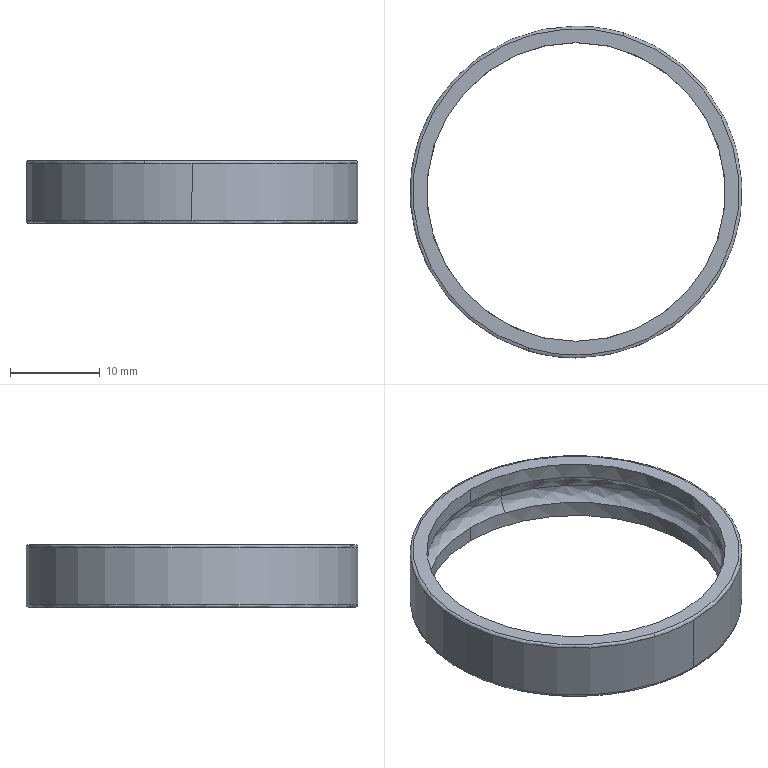Part | SolidWorks | features BaseBody 1 | 1 solid | 16 faces | box 37 x 37 x 7 mm | volume 1192 mm3 | spline 8 | cylinder 6 | plane 2 | commonest cylinder face diameters 33.3 x4 37 x2
STEP:
#1=CARTESIAN_POINT('',(518.571,7.238,245.844));
#2=VERTEX_POINT('',#1);
#3=CARTESIAN_POINT('',(513.262,8.017,245.844));
#4=VERTEX_POINT('',#3);
#5=CARTESIAN_POINT('',(513.262,-10.483,245.844));
#6=DIRECTION('',(0.000000004,-0.00000001,1.));
#7=DIRECTION('',(0.,-1.,-0.00000001));
#8=AXIS2_PLACEMENT_3D('',#5,#6,#7);
#9=CIRCLE('',#8,18.5);
#10=EDGE_CURVE('',#2,#4,#9,.T.);
#11=ORIENTED_EDGE('',*,*,#10,.F.);
#12=CARTESIAN_POINT('',(518.485,6.951,245.544));
#13=VERTEX_POINT('',#12);
#14=CARTESIAN_POINT('',(518.485,6.951,245.844));
#15=DIRECTION('',(-0.9579,0.287,0.000000007));
#16=DIRECTION('',(0.287,0.9579,0.000000008));
#17=AXIS2_PLACEMENT_3D('',#14,#15,#16);
#18=CIRCLE('',#17,0.3);
#19=EDGE_CURVE('',#2,#13,#18,.T.);
#20=ORIENTED_EDGE('',*,*,#19,.T.);
#21=CARTESIAN_POINT('',(508.038,-27.918,245.544));
#22=VERTEX_POINT('',#21);
#23=CARTESIAN_POINT('',(518.485,6.951,245.544));
#24=CARTESIAN_POINT('',(483.617,17.398,245.544));
#25=CARTESIAN_POINT('',(473.169,-17.47,245.544));
#26=CARTESIAN_POINT('',(508.038,-27.918,245.544));
#27=(BOUNDED_CURVE()B_SPLINE_CURVE(3,(#23,#24,#25,#26),.UNSPECIFIED.,.F.,.F.)B_SPLINE_CURVE_WITH_KNOTS((4,4),(0.,1.),.UNSPECIFIED.)CURVE()GEOMETRIC_REPRESENTATION_ITEM()RATIONAL_B_SPLINE_CURVE((1.,0.3333,0.3333,1.))REPRESENTATION_ITEM(''));
#28=EDGE_CURVE('',#13,#22,#27,.T.);
#29=ORIENTED_EDGE('',*,*,#28,.T.);
#30=CARTESIAN_POINT('',(507.952,-28.205,245.844));
#31=VERTEX_POINT('',#30);
#32=CARTESIAN_POINT('',(508.038,-27.918,245.844));
#33=DIRECTION('',(0.9579,-0.287,-0.000000007));
#34=DIRECTION('',(-0.287,-0.9579,-0.000000008));
#35=AXIS2_PLACEMENT_3D('',#32,#33,#34);
#36=CIRCLE('',#35,0.3);
#37=EDGE_CURVE('',#31,#22,#36,.T.);
#38=ORIENTED_EDGE('',*,*,#37,.F.);
#39=CARTESIAN_POINT('',(513.262,-10.483,245.844));
#40=DIRECTION('',(0.000000004,-0.00000001,1.));
#41=DIRECTION('',(0.,-1.,-0.00000001));
#42=AXIS2_PLACEMENT_3D('',#39,#40,#41);
#43=CIRCLE('',#42,18.5);
#44=EDGE_CURVE('',#4,#31,#43,.T.);
#45=ORIENTED_EDGE('',*,*,#44,.F.);
#46=EDGE_LOOP('',(#11,#20,#29,#38,#45));
#47=FACE_OUTER_BOUND('',#46,.T.);
#48=CARTESIAN_POINT('',(518.571,7.238,245.844));
#49=CARTESIAN_POINT('',(483.128,17.858,245.844));
#50=CARTESIAN_POINT('',(472.508,-17.585,245.844));
#51=CARTESIAN_POINT('',(507.952,-28.205,245.844));
#52=CARTESIAN_POINT('',(518.571,7.238,245.669));
#53=CARTESIAN_POINT('',(483.128,17.858,245.669));
#54=CARTESIAN_POINT('',(472.508,-17.585,245.669));
#55=CARTESIAN_POINT('',(507.952,-28.205,245.669));
#56=CARTESIAN_POINT('',(518.536,7.119,245.544));
#57=CARTESIAN_POINT('',(483.331,17.668,245.544));
#58=CARTESIAN_POINT('',(472.782,-17.537,245.544));
#59=CARTESIAN_POINT('',(507.987,-28.086,245.544));
#60=CARTESIAN_POINT('',(518.485,6.951,245.544));
#61=CARTESIAN_POINT('',(483.617,17.398,245.544));
#62=CARTESIAN_POINT('',(473.169,-17.47,245.544));
#63=CARTESIAN_POINT('',(508.038,-27.918,245.544));
#64=(BOUNDED_SURFACE()B_SPLINE_SURFACE(3,3,((#48,#49,#50,#51),(#52,#53,#54,#55),(#56,#57,#58,#59),(#60,#61,#62,#63)),.UNSPECIFIED.,.F.,.F.,.F.)B_SPLINE_SURFACE_WITH_KNOTS((4,4),(4,4),(0.,1.),(0.,1.),.UNSPECIFIED.)GEOMETRIC_REPRESENTATION_ITEM()RATIONAL_B_SPLINE_SURFACE(((1.,0.3333,0.3333,1.),(0.8047,0.2682,0.2682,0.8047),(0.8047,0.2682,0.2682,0.8047),(1.,0.3333,0.3333,1.)))REPRESENTATION_ITEM('')SURFACE());
#65=ADVANCED_FACE('',(#47),#64,.T.);
#66=CARTESIAN_POINT('',(508.038,-27.918,252.544));
#67=VERTEX_POINT('',#66);
#68=CARTESIAN_POINT('',(518.485,6.951,252.544));
#69=VERTEX_POINT('',#68);
#70=CARTESIAN_POINT('',(508.038,-27.918,252.544));
#71=CARTESIAN_POINT('',(473.169,-17.47,252.544));
#72=CARTESIAN_POINT('',(483.617,17.398,252.544));
#73=CARTESIAN_POINT('',(518.485,6.951,252.544));
#74=(BOUNDED_CURVE()B_SPLINE_CURVE(3,(#70,#71,#72,#73),.UNSPECIFIED.,.F.,.F.)B_SPLINE_CURVE_WITH_KNOTS((4,4),(0.,1.),.UNSPECIFIED.)CURVE()GEOMETRIC_REPRESENTATION_ITEM()RATIONAL_B_SPLINE_CURVE((1.,0.3333,0.3333,1.))REPRESENTATION_ITEM(''));
#75=EDGE_CURVE('',#67,#69,#74,.T.);
#76=ORIENTED_EDGE('',*,*,#75,.T.);
#77=CARTESIAN_POINT('',(518.571,7.238,252.244));
#78=VERTEX_POINT('',#77);
#79=CARTESIAN_POINT('',(518.485,6.951,252.244));
#80=DIRECTION('',(-0.9579,0.287,0.000000007));
#81=DIRECTION('',(0.287,0.9579,0.000000008));
#82=AXIS2_PLACEMENT_3D('',#79,#80,#81);
#83=CIRCLE('',#82,0.3);
#84=EDGE_CURVE('',#69,#78,#83,.T.);
#85=ORIENTED_EDGE('',*,*,#84,.T.);
#86=CARTESIAN_POINT('',(513.262,8.017,252.244));
#87=VERTEX_POINT('',#86);
#88=CARTESIAN_POINT('',(513.262,-10.483,252.244));
#89=DIRECTION('',(-0.000000004,0.00000001,-1.));
#90=DIRECTION('',(0.,-1.,-0.00000001));
#91=AXIS2_PLACEMENT_3D('',#88,#89,#90);
#92=CIRCLE('',#91,18.5);
#93=EDGE_CURVE('',#87,#78,#92,.T.);
#94=ORIENTED_EDGE('',*,*,#93,.F.);
#95=CARTESIAN_POINT('',(507.952,-28.205,252.244));
#96=VERTEX_POINT('',#95);
#97=CARTESIAN_POINT('',(513.262,-10.483,252.244));
#98=DIRECTION('',(-0.000000004,0.00000001,-1.));
#99=DIRECTION('',(0.,-1.,-0.00000001));
#100=AXIS2_PLACEMENT_3D('',#97,#98,#99);
#101=CIRCLE('',#100,18.5);
#102=EDGE_CURVE('',#96,#87,#101,.T.);
#103=ORIENTED_EDGE('',*,*,#102,.F.);
#104=CARTESIAN_POINT('',(508.038,-27.918,252.244));
#105=DIRECTION('',(0.9579,-0.287,-0.000000007));
#106=DIRECTION('',(-0.287,-0.9579,-0.000000008));
#107=AXIS2_PLACEMENT_3D('',#104,#105,#106);
#108=CIRCLE('',#107,0.3);
#109=EDGE_CURVE('',#67,#96,#108,.T.);
#110=ORIENTED_EDGE('',*,*,#109,.F.);
#111=EDGE_LOOP('',(#76,#85,#94,#103,#110));
#112=FACE_OUTER_BOUND('',#111,.T.);
#113=CARTESIAN_POINT('',(518.485,6.951,252.544));
#114=CARTESIAN_POINT('',(483.617,17.398,252.544));
#115=CARTESIAN_POINT('',(473.169,-17.47,252.544));
#116=CARTESIAN_POINT('',(508.038,-27.918,252.544));
#117=CARTESIAN_POINT('',(518.536,7.119,252.544));
#118=CARTESIAN_POINT('',(483.331,17.668,252.544));
#119=CARTESIAN_POINT('',(472.782,-17.537,252.544));
#120=CARTESIAN_POINT('',(507.987,-28.086,252.544));
#121=CARTESIAN_POINT('',(518.571,7.238,252.42));
#122=CARTESIAN_POINT('',(483.128,17.858,252.42));
#123=CARTESIAN_POINT('',(472.508,-17.585,252.42));
#124=CARTESIAN_POINT('',(507.952,-28.205,252.42));
#125=CARTESIAN_POINT('',(518.571,7.238,252.244));
#126=CARTESIAN_POINT('',(483.128,17.858,252.244));
#127=CARTESIAN_POINT('',(472.508,-17.585,252.244));
#128=CARTESIAN_POINT('',(507.952,-28.205,252.244));
#129=(BOUNDED_SURFACE()B_SPLINE_SURFACE(3,3,((#113,#114,#115,#116),(#117,#118,#119,#120),(#121,#122,#123,#124),(#125,#126,#127,#128)),.UNSPECIFIED.,.F.,.F.,.T.)B_SPLINE_SURFACE_WITH_KNOTS((4,4),(4,4),(0.,1.),(0.,1.),.UNSPECIFIED.)GEOMETRIC_REPRESENTATION_ITEM()RATIONAL_B_SPLINE_SURFACE(((1.,0.3333,0.3333,1.),(0.8047,0.2682,0.2682,0.8047),(0.8047,0.2682,0.2682,0.8047),(1.,0.3333,0.3333,1.)))REPRESENTATION_ITEM('')SURFACE());
#130=ADVANCED_FACE('',(#112),#129,.T.);
#131=CARTESIAN_POINT('',(513.262,-27.133,250.768));
#132=VERTEX_POINT('',#131);
#133=CARTESIAN_POINT('',(518.04,5.466,250.768));
#134=VERTEX_POINT('',#133);
#135=CARTESIAN_POINT('',(513.262,-10.483,250.768));
#136=DIRECTION('',(0.000000004,-0.00000001,1.));
#137=DIRECTION('',(0.,-1.,-0.00000001));
#138=AXIS2_PLACEMENT_3D('',#135,#136,#137);
#139=CIRCLE('',#138,16.65);
#140=EDGE_CURVE('',#132,#134,#139,.T.);
#141=ORIENTED_EDGE('',*,*,#140,.T.);
#142=CARTESIAN_POINT('',(518.299,6.328,249.044));
#143=VERTEX_POINT('',#142);
#144=CARTESIAN_POINT('',(517.696,4.317,249.044));
#145=DIRECTION('',(-0.9579,0.287,0.000000007));
#146=DIRECTION('',(0.287,0.9579,0.000000008));
#147=AXIS2_PLACEMENT_3D('',#144,#145,#146);
#148=CIRCLE('',#147,2.1);
#149=EDGE_CURVE('',#134,#143,#148,.T.);
#150=ORIENTED_EDGE('',*,*,#149,.T.);
#151=CARTESIAN_POINT('',(508.224,-27.295,249.044));
#152=VERTEX_POINT('',#151);
#153=CARTESIAN_POINT('',(513.262,-10.483,249.044));
#154=DIRECTION('',(0.000000004,-0.00000001,1.));
#155=DIRECTION('',(-0.287,-0.9579,-0.000000008));
#156=AXIS2_PLACEMENT_3D('',#153,#154,#155);
#157=CIRCLE('',#156,17.55);
#158=EDGE_CURVE('',#152,#143,#157,.T.);
#159=ORIENTED_EDGE('',*,*,#158,.F.);
#160=CARTESIAN_POINT('',(508.483,-26.433,250.768));
#161=VERTEX_POINT('',#160);
#162=CARTESIAN_POINT('',(508.827,-25.283,249.044));
#163=DIRECTION('',(0.9579,-0.287,-0.000000007));
#164=DIRECTION('',(-0.287,-0.9579,-0.000000008));
#165=AXIS2_PLACEMENT_3D('',#162,#163,#164);
#166=CIRCLE('',#165,2.1);
#167=EDGE_CURVE('',#161,#152,#166,.T.);
#168=ORIENTED_EDGE('',*,*,#167,.F.);
#169=CARTESIAN_POINT('',(513.262,-10.483,250.768));
#170=DIRECTION('',(0.000000004,-0.00000001,1.));
#171=DIRECTION('',(0.,-1.,-0.00000001));
#172=AXIS2_PLACEMENT_3D('',#169,#170,#171);
#173=CIRCLE('',#172,16.65);
#174=EDGE_CURVE('',#161,#132,#173,.T.);
#175=ORIENTED_EDGE('',*,*,#174,.T.);
#176=EDGE_LOOP('',(#141,#150,#159,#168,#175));
#177=FACE_OUTER_BOUND('',#176,.T.);
#178=CARTESIAN_POINT('',(508.483,-26.433,250.768));
#179=CARTESIAN_POINT('',(540.381,-35.991,250.768));
#180=CARTESIAN_POINT('',(549.939,-4.092,250.768));
#181=CARTESIAN_POINT('',(518.04,5.466,250.768));
#182=CARTESIAN_POINT('',(508.317,-26.984,250.367));
#183=CARTESIAN_POINT('',(541.319,-36.872,250.367));
#184=CARTESIAN_POINT('',(551.207,-3.871,250.367));
#185=CARTESIAN_POINT('',(518.206,6.017,250.367));
#186=CARTESIAN_POINT('',(508.224,-27.295,249.745));
#187=CARTESIAN_POINT('',(541.847,-37.369,249.745));
#188=CARTESIAN_POINT('',(551.922,-3.746,249.745));
#189=CARTESIAN_POINT('',(518.299,6.328,249.745));
#190=CARTESIAN_POINT('',(508.224,-27.295,249.044));
#191=CARTESIAN_POINT('',(541.847,-37.369,249.044));
#192=CARTESIAN_POINT('',(551.922,-3.746,249.044));
#193=CARTESIAN_POINT('',(518.299,6.328,249.044));
#194=(BOUNDED_SURFACE()B_SPLINE_SURFACE(3,3,((#178,#179,#180,#181),(#182,#183,#184,#185),(#186,#187,#188,#189),(#190,#191,#192,#193)),.UNSPECIFIED.,.F.,.F.,.F.)B_SPLINE_SURFACE_WITH_KNOTS((4,4),(4,4),(0.,1.),(0.,1.),.UNSPECIFIED.)GEOMETRIC_REPRESENTATION_ITEM()RATIONAL_B_SPLINE_SURFACE(((1.,0.3333,0.3333,1.),(0.9243,0.3081,0.3081,0.9243),(0.9243,0.3081,0.3081,0.9243),(1.,0.3333,0.3333,1.)))REPRESENTATION_ITEM('')SURFACE());
#195=ADVANCED_FACE('',(#177),#194,.F.);
#196=ORIENTED_EDGE('',*,*,#158,.T.);
#197=CARTESIAN_POINT('',(518.04,5.466,247.321));
#198=VERTEX_POINT('',#197);
#199=CARTESIAN_POINT('',(517.696,4.317,249.044));
#200=DIRECTION('',(-0.9579,0.287,0.000000007));
#201=DIRECTION('',(0.287,0.9579,0.000000008));
#202=AXIS2_PLACEMENT_3D('',#199,#200,#201);
#203=CIRCLE('',#202,2.1);
#204=EDGE_CURVE('',#143,#198,#203,.T.);
#205=ORIENTED_EDGE('',*,*,#204,.T.);
#206=CARTESIAN_POINT('',(513.262,-27.133,247.321));
#207=VERTEX_POINT('',#206);
#208=CARTESIAN_POINT('',(513.262,-10.483,247.321));
#209=DIRECTION('',(-0.000000004,0.00000001,-1.));
#210=DIRECTION('',(0.,-1.,-0.00000001));
#211=AXIS2_PLACEMENT_3D('',#208,#209,#210);
#212=CIRCLE('',#211,16.65);
#213=EDGE_CURVE('',#198,#207,#212,.T.);
#214=ORIENTED_EDGE('',*,*,#213,.T.);
#215=CARTESIAN_POINT('',(508.483,-26.433,247.321));
#216=VERTEX_POINT('',#215);
#217=CARTESIAN_POINT('',(513.262,-10.483,247.321));
#218=DIRECTION('',(-0.000000004,0.00000001,-1.));
#219=DIRECTION('',(0.,-1.,-0.00000001));
#220=AXIS2_PLACEMENT_3D('',#217,#218,#219);
#221=CIRCLE('',#220,16.65);
#222=EDGE_CURVE('',#207,#216,#221,.T.);
#223=ORIENTED_EDGE('',*,*,#222,.T.);
#224=CARTESIAN_POINT('',(508.827,-25.283,249.044));
#225=DIRECTION('',(0.9579,-0.287,-0.000000007));
#226=DIRECTION('',(-0.287,-0.9579,-0.000000008));
#227=AXIS2_PLACEMENT_3D('',#224,#225,#226);
#228=CIRCLE('',#227,2.1);
#229=EDGE_CURVE('',#152,#216,#228,.T.);
#230=ORIENTED_EDGE('',*,*,#229,.F.);
#231=EDGE_LOOP('',(#196,#205,#214,#223,#230));
#232=FACE_OUTER_BOUND('',#231,.T.);
#233=CARTESIAN_POINT('',(508.224,-27.295,249.044));
#234=CARTESIAN_POINT('',(541.847,-37.369,249.044));
#235=CARTESIAN_POINT('',(551.922,-3.746,249.044));
#236=CARTESIAN_POINT('',(518.299,6.328,249.044));
#237=CARTESIAN_POINT('',(508.224,-27.295,248.343));
#238=CARTESIAN_POINT('',(541.847,-37.369,248.343));
#239=CARTESIAN_POINT('',(551.922,-3.746,248.343));
#240=CARTESIAN_POINT('',(518.299,6.328,248.343));
#241=CARTESIAN_POINT('',(508.317,-26.984,247.722));
#242=CARTESIAN_POINT('',(541.319,-36.872,247.722));
#243=CARTESIAN_POINT('',(551.207,-3.871,247.722));
#244=CARTESIAN_POINT('',(518.206,6.017,247.722));
#245=CARTESIAN_POINT('',(508.483,-26.433,247.321));
#246=CARTESIAN_POINT('',(540.381,-35.991,247.321));
#247=CARTESIAN_POINT('',(549.939,-4.092,247.321));
#248=CARTESIAN_POINT('',(518.04,5.466,247.321));
#249=(BOUNDED_SURFACE()B_SPLINE_SURFACE(3,3,((#233,#234,#235,#236),(#237,#238,#239,#240),(#241,#242,#243,#244),(#245,#246,#247,#248)),.UNSPECIFIED.,.F.,.F.,.F.)B_SPLINE_SURFACE_WITH_KNOTS((4,4),(4,4),(0.,1.),(0.,1.),.UNSPECIFIED.)GEOMETRIC_REPRESENTATION_ITEM()RATIONAL_B_SPLINE_SURFACE(((1.,0.3333,0.3333,1.),(0.9243,0.3081,0.3081,0.9243),(0.9243,0.3081,0.3081,0.9243),(1.,0.3333,0.3333,1.)))REPRESENTATION_ITEM('')SURFACE());
#250=ADVANCED_FACE('',(#232),#249,.F.);
#251=CARTESIAN_POINT('',(513.262,-28.983,245.844));
#252=VERTEX_POINT('',#251);
#253=CARTESIAN_POINT('',(513.262,-10.483,245.844));
#254=DIRECTION('',(0.000000004,-0.00000001,1.));
#255=DIRECTION('',(0.,-1.,-0.00000001));
#256=AXIS2_PLACEMENT_3D('',#253,#254,#255);
#257=CIRCLE('',#256,18.5);
#258=EDGE_CURVE('',#252,#2,#257,.T.);
#259=ORIENTED_EDGE('',*,*,#258,.T.);
#260=ORIENTED_EDGE('',*,*,#10,.T.);
#261=CARTESIAN_POINT('',(513.262,8.017,249.044));
#262=DIRECTION('',(0.000000004,-0.00000001,1.));
#263=VECTOR('',#262,1000.);
#264=LINE('',#261,#263);
#265=EDGE_CURVE('',#4,#87,#264,.T.);
#266=ORIENTED_EDGE('',*,*,#265,.T.);
#267=ORIENTED_EDGE('',*,*,#93,.T.);
#268=CARTESIAN_POINT('',(513.262,-28.983,252.244));
#269=VERTEX_POINT('',#268);
#270=CARTESIAN_POINT('',(513.262,-10.483,252.244));
#271=DIRECTION('',(-0.000000004,0.00000001,-1.));
#272=DIRECTION('',(0.,-1.,-0.00000001));
#273=AXIS2_PLACEMENT_3D('',#270,#271,#272);
#274=CIRCLE('',#273,18.5);
#275=EDGE_CURVE('',#78,#269,#274,.T.);
#276=ORIENTED_EDGE('',*,*,#275,.T.);
#277=CARTESIAN_POINT('',(513.262,-28.983,249.044));
#278=DIRECTION('',(0.000000004,-0.00000001,1.));
#279=VECTOR('',#278,1000.);
#280=LINE('',#277,#279);
#281=EDGE_CURVE('',#252,#269,#280,.T.);
#282=ORIENTED_EDGE('',*,*,#281,.F.);
#283=EDGE_LOOP('',(#259,#260,#266,#267,#276,#282));
#284=FACE_OUTER_BOUND('',#283,.T.);
#285=CARTESIAN_POINT('',(513.262,-10.483,249.044));
#286=DIRECTION('',(0.000000004,-0.00000001,1.));
#287=DIRECTION('',(0.,-1.,-0.00000001));
#288=AXIS2_PLACEMENT_3D('',#285,#286,#287);
#289=CYLINDRICAL_SURFACE('',#288,18.5);
#290=ADVANCED_FACE('',(#284),#289,.T.);
#291=CARTESIAN_POINT('',(513.262,6.167,245.544));
#292=VERTEX_POINT('',#291);
#293=CARTESIAN_POINT('',(513.262,-27.133,245.544));
#294=VERTEX_POINT('',#293);
#295=CARTESIAN_POINT('',(513.262,-10.483,245.544));
#296=DIRECTION('',(0.000000004,-0.00000001,1.));
#297=DIRECTION('',(0.,-1.,-0.00000001));
#298=AXIS2_PLACEMENT_3D('',#295,#296,#297);
#299=CIRCLE('',#298,16.65);
#300=EDGE_CURVE('',#292,#294,#299,.T.);
#301=ORIENTED_EDGE('',*,*,#300,.F.);
#302=CARTESIAN_POINT('',(513.262,6.167,247.321));
#303=VERTEX_POINT('',#302);
#304=CARTESIAN_POINT('',(513.262,6.167,246.433));
#305=DIRECTION('',(0.000000004,-0.00000001,1.));
#306=VECTOR('',#305,1000.);
#307=LINE('',#304,#306);
#308=EDGE_CURVE('',#292,#303,#307,.T.);
#309=ORIENTED_EDGE('',*,*,#308,.T.);
#310=CARTESIAN_POINT('',(513.262,-10.483,247.321));
#311=DIRECTION('',(-0.000000004,0.00000001,-1.));
#312=DIRECTION('',(0.,-1.,-0.00000001));
#313=AXIS2_PLACEMENT_3D('',#310,#311,#312);
#314=CIRCLE('',#313,16.65);
#315=EDGE_CURVE('',#216,#303,#314,.T.);
#316=ORIENTED_EDGE('',*,*,#315,.F.);
#317=ORIENTED_EDGE('',*,*,#222,.F.);
#318=CARTESIAN_POINT('',(513.262,-27.133,246.433));
#319=DIRECTION('',(0.000000004,-0.00000001,1.));
#320=VECTOR('',#319,1000.);
#321=LINE('',#318,#320);
#322=EDGE_CURVE('',#294,#207,#321,.T.);
#323=ORIENTED_EDGE('',*,*,#322,.F.);
#324=EDGE_LOOP('',(#301,#309,#316,#317,#323));
#325=FACE_OUTER_BOUND('',#324,.T.);
#326=CARTESIAN_POINT('',(513.262,-10.483,246.433));
#327=DIRECTION('',(0.000000004,-0.00000001,1.));
#328=DIRECTION('',(0.,-1.,-0.00000001));
#329=AXIS2_PLACEMENT_3D('',#326,#327,#328);
#330=CYLINDRICAL_SURFACE('',#329,16.65);
#331=ADVANCED_FACE('',(#325),#330,.F.);
#332=CARTESIAN_POINT('',(513.262,6.167,250.768));
#333=VERTEX_POINT('',#332);
#334=CARTESIAN_POINT('',(513.262,-10.483,250.768));
#335=DIRECTION('',(0.000000004,-0.00000001,1.));
#336=DIRECTION('',(0.,-1.,-0.00000001));
#337=AXIS2_PLACEMENT_3D('',#334,#335,#336);
#338=CIRCLE('',#337,16.65);
#339=EDGE_CURVE('',#333,#161,#338,.T.);
#340=ORIENTED_EDGE('',*,*,#339,.F.);
#341=CARTESIAN_POINT('',(513.262,6.167,252.544));
#342=VERTEX_POINT('',#341);
#343=CARTESIAN_POINT('',(513.262,6.167,251.656));
#344=DIRECTION('',(0.000000004,-0.00000001,1.));
#345=VECTOR('',#344,1000.);
#346=LINE('',#343,#345);
#347=EDGE_CURVE('',#333,#342,#346,.T.);
#348=ORIENTED_EDGE('',*,*,#347,.T.);
#349=CARTESIAN_POINT('',(513.262,-27.133,252.544));
#350=VERTEX_POINT('',#349);
#351=CARTESIAN_POINT('',(513.262,-10.483,252.544));
#352=DIRECTION('',(-0.000000004,0.00000001,-1.));
#353=DIRECTION('',(0.,-1.,-0.00000001));
#354=AXIS2_PLACEMENT_3D('',#351,#352,#353);
#355=CIRCLE('',#354,16.65);
#356=EDGE_CURVE('',#350,#342,#355,.T.);
#357=ORIENTED_EDGE('',*,*,#356,.F.);
#358=CARTESIAN_POINT('',(513.262,-27.133,251.656));
#359=DIRECTION('',(0.000000004,-0.00000001,1.));
#360=VECTOR('',#359,1000.);
#361=LINE('',#358,#360);
#362=EDGE_CURVE('',#132,#350,#361,.T.);
#363=ORIENTED_EDGE('',*,*,#362,.F.);
#364=ORIENTED_EDGE('',*,*,#174,.F.);
#365=EDGE_LOOP('',(#340,#348,#357,#363,#364));
#366=FACE_OUTER_BOUND('',#365,.T.);
#367=CARTESIAN_POINT('',(513.262,-10.483,251.656));
#368=DIRECTION('',(0.000000004,-0.00000001,1.));
#369=DIRECTION('',(0.,-1.,-0.00000001));
#370=AXIS2_PLACEMENT_3D('',#367,#368,#369);
#371=CYLINDRICAL_SURFACE('',#370,16.65);
#372=ADVANCED_FACE('',(#366),#371,.F.);
#373=ORIENTED_EDGE('',*,*,#204,.F.);
#374=CARTESIAN_POINT('',(513.262,-10.483,249.044));
#375=DIRECTION('',(0.000000004,-0.00000001,1.));
#376=DIRECTION('',(-0.287,-0.9579,-0.000000008));
#377=AXIS2_PLACEMENT_3D('',#374,#375,#376);
#378=CIRCLE('',#377,17.55);
#379=EDGE_CURVE('',#143,#152,#378,.T.);
#380=ORIENTED_EDGE('',*,*,#379,.T.);
#381=ORIENTED_EDGE('',*,*,#229,.T.);
#382=ORIENTED_EDGE('',*,*,#315,.T.);
#383=CARTESIAN_POINT('',(513.262,-10.483,247.321));
#384=DIRECTION('',(-0.000000004,0.00000001,-1.));
#385=DIRECTION('',(0.,-1.,-0.00000001));
#386=AXIS2_PLACEMENT_3D('',#383,#384,#385);
#387=CIRCLE('',#386,16.65);
#388=EDGE_CURVE('',#303,#198,#387,.T.);
#389=ORIENTED_EDGE('',*,*,#388,.T.);
#390=EDGE_LOOP('',(#373,#380,#381,#382,#389));
#391=FACE_OUTER_BOUND('',#390,.T.);
#392=CARTESIAN_POINT('',(518.299,6.328,249.044));
#393=CARTESIAN_POINT('',(484.676,16.403,249.044));
#394=CARTESIAN_POINT('',(474.601,-17.22,249.044));
#395=CARTESIAN_POINT('',(508.224,-27.295,249.044));
#396=CARTESIAN_POINT('',(518.299,6.328,248.343));
#397=CARTESIAN_POINT('',(484.676,16.403,248.343));
#398=CARTESIAN_POINT('',(474.601,-17.22,248.343));
#399=CARTESIAN_POINT('',(508.224,-27.295,248.343));
#400=CARTESIAN_POINT('',(518.206,6.017,247.722));
#401=CARTESIAN_POINT('',(485.204,15.905,247.722));
#402=CARTESIAN_POINT('',(475.316,-17.096,247.722));
#403=CARTESIAN_POINT('',(508.317,-26.984,247.722));
#404=CARTESIAN_POINT('',(518.04,5.466,247.321));
#405=CARTESIAN_POINT('',(486.142,15.024,247.321));
#406=CARTESIAN_POINT('',(476.584,-16.875,247.321));
#407=CARTESIAN_POINT('',(508.483,-26.433,247.321));
#408=(BOUNDED_SURFACE()B_SPLINE_SURFACE(3,3,((#392,#393,#394,#395),(#396,#397,#398,#399),(#400,#401,#402,#403),(#404,#405,#406,#407)),.UNSPECIFIED.,.F.,.F.,.F.)B_SPLINE_SURFACE_WITH_KNOTS((4,4),(4,4),(0.,1.),(0.,1.),.UNSPECIFIED.)GEOMETRIC_REPRESENTATION_ITEM()RATIONAL_B_SPLINE_SURFACE(((1.,0.3333,0.3333,1.),(0.9243,0.3081,0.3081,0.9243),(0.9243,0.3081,0.3081,0.9243),(1.,0.3333,0.3333,1.)))REPRESENTATION_ITEM('')SURFACE());
#409=ADVANCED_FACE('',(#391),#408,.F.);
#410=ORIENTED_EDGE('',*,*,#265,.F.);
#411=ORIENTED_EDGE('',*,*,#44,.T.);
#412=CARTESIAN_POINT('',(513.262,-10.483,245.844));
#413=DIRECTION('',(0.000000004,-0.00000001,1.));
#414=DIRECTION('',(0.,-1.,-0.00000001));
#415=AXIS2_PLACEMENT_3D('',#412,#413,#414);
#416=CIRCLE('',#415,18.5);
#417=EDGE_CURVE('',#31,#252,#416,.T.);
#418=ORIENTED_EDGE('',*,*,#417,.T.);
#419=ORIENTED_EDGE('',*,*,#281,.T.);
#420=CARTESIAN_POINT('',(513.262,-10.483,252.244));
#421=DIRECTION('',(-0.000000004,0.00000001,-1.));
#422=DIRECTION('',(0.,-1.,-0.00000001));
#423=AXIS2_PLACEMENT_3D('',#420,#421,#422);
#424=CIRCLE('',#423,18.5);
#425=EDGE_CURVE('',#269,#96,#424,.T.);
#426=ORIENTED_EDGE('',*,*,#425,.T.);
#427=ORIENTED_EDGE('',*,*,#102,.T.);
#428=EDGE_LOOP('',(#410,#411,#418,#419,#426,#427));
#429=FACE_OUTER_BOUND('',#428,.T.);
#430=CARTESIAN_POINT('',(513.262,-10.483,249.044));
#431=DIRECTION('',(0.000000004,-0.00000001,1.));
#432=DIRECTION('',(0.,-1.,-0.00000001));
#433=AXIS2_PLACEMENT_3D('',#430,#431,#432);
#434=CYLINDRICAL_SURFACE('',#433,18.5);
#435=ADVANCED_FACE('',(#429),#434,.T.);
#436=ORIENTED_EDGE('',*,*,#19,.F.);
#437=ORIENTED_EDGE('',*,*,#258,.F.);
#438=ORIENTED_EDGE('',*,*,#417,.F.);
#439=ORIENTED_EDGE('',*,*,#37,.T.);
#440=CARTESIAN_POINT('',(518.485,6.951,245.544));
#441=CARTESIAN_POINT('',(519.018,6.791,245.544));
#442=CARTESIAN_POINT('',(519.804,6.516,245.544));
#443=CARTESIAN_POINT('',(520.695,6.133,245.544));
#444=CARTESIAN_POINT('',(521.135,5.926,245.544));
#445=CARTESIAN_POINT('',(521.353,5.819,245.544));
#446=CARTESIAN_POINT('',(521.446,5.772,245.544));
#447=CARTESIAN_POINT('',(521.509,5.741,245.544));
#448=CARTESIAN_POINT('',(521.538,5.726,245.544));
#449=CARTESIAN_POINT('',(522.095,5.44,245.544));
#450=CARTESIAN_POINT('',(522.86,5.,245.544));
#451=CARTESIAN_POINT('',(523.711,4.423,245.544));
#452=CARTESIAN_POINT('',(524.127,4.119,245.544));
#453=CARTESIAN_POINT('',(524.332,3.963,245.544));
#454=CARTESIAN_POINT('',(524.42,3.895,245.544));
#455=CARTESIAN_POINT('',(524.478,3.85,245.544));
#456=CARTESIAN_POINT('',(524.506,3.828,245.544));
#457=CARTESIAN_POINT('',(525.019,3.423,245.544));
#458=CARTESIAN_POINT('',(525.71,2.818,245.544));
#459=CARTESIAN_POINT('',(526.461,2.054,245.544));
#460=CARTESIAN_POINT('',(526.822,1.657,245.544));
#461=CARTESIAN_POINT('',(526.974,1.484,245.544));
#462=CARTESIAN_POINT('',(527.074,1.368,245.544));
#463=CARTESIAN_POINT('',(527.123,1.311,245.544));
#464=CARTESIAN_POINT('',(527.984,0.2903,245.544));
#465=CARTESIAN_POINT('',(528.687,-0.7435,245.544));
#466=CARTESIAN_POINT('',(529.581,-2.402,245.544));
#467=CARTESIAN_POINT('',(529.983,-3.25,245.544));
#468=CARTESIAN_POINT('',(530.374,-4.272,245.544));
#469=CARTESIAN_POINT('',(530.55,-4.791,245.544));
#470=CARTESIAN_POINT('',(530.621,-5.015,245.544));
#471=CARTESIAN_POINT('',(530.667,-5.165,245.544));
#472=CARTESIAN_POINT('',(530.691,-5.242,245.544));
#473=CARTESIAN_POINT('',(530.887,-5.905,245.544));
#474=CARTESIAN_POINT('',(531.103,-6.798,245.544));
#475=CARTESIAN_POINT('',(531.276,-7.855,245.544));
#476=CARTESIAN_POINT('',(531.342,-8.388,245.544));
#477=CARTESIAN_POINT('',(531.37,-8.655,245.544));
#478=CARTESIAN_POINT('',(531.381,-8.77,245.544));
#479=CARTESIAN_POINT('',(531.388,-8.846,245.544));
#480=CARTESIAN_POINT('',(531.391,-8.886,245.544));
#481=CARTESIAN_POINT('',(531.445,-9.511,245.544));
#482=CARTESIAN_POINT('',(531.478,-10.392,245.544));
#483=CARTESIAN_POINT('',(531.442,-11.42,245.544));
#484=CARTESIAN_POINT('',(531.405,-11.934,245.544));
#485=CARTESIAN_POINT('',(531.382,-12.191,245.544));
#486=CARTESIAN_POINT('',(531.371,-12.301,245.544));
#487=CARTESIAN_POINT('',(531.363,-12.374,245.544));
#488=CARTESIAN_POINT('',(531.359,-12.413,245.544));
#489=CARTESIAN_POINT('',(531.235,-13.554,245.544));
#490=CARTESIAN_POINT('',(531.015,-14.641,245.544));
#491=CARTESIAN_POINT('',(530.536,-16.24,245.544));
#492=CARTESIAN_POINT('',(530.261,-17.026,245.544));
#493=CARTESIAN_POINT('',(529.878,-17.917,245.544));
#494=CARTESIAN_POINT('',(529.671,-18.357,245.544));
#495=CARTESIAN_POINT('',(529.564,-18.575,245.544));
#496=CARTESIAN_POINT('',(529.517,-18.668,245.544));
#497=CARTESIAN_POINT('',(529.486,-18.73,245.544));
#498=CARTESIAN_POINT('',(529.471,-18.76,245.544));
#499=CARTESIAN_POINT('',(529.185,-19.317,245.544));
#500=CARTESIAN_POINT('',(528.745,-20.082,245.544));
#501=CARTESIAN_POINT('',(528.168,-20.933,245.544));
#502=CARTESIAN_POINT('',(527.864,-21.349,245.544));
#503=CARTESIAN_POINT('',(527.708,-21.554,245.544));
#504=CARTESIAN_POINT('',(527.64,-21.642,245.544));
#505=CARTESIAN_POINT('',(527.594,-21.7,245.544));
#506=CARTESIAN_POINT('',(527.573,-21.728,245.544));
#507=CARTESIAN_POINT('',(527.168,-22.241,245.544));
#508=CARTESIAN_POINT('',(526.563,-22.932,245.544));
#509=CARTESIAN_POINT('',(525.799,-23.683,245.544));
#510=CARTESIAN_POINT('',(525.402,-24.044,245.544));
#511=CARTESIAN_POINT('',(525.229,-24.196,245.544));
#512=CARTESIAN_POINT('',(525.113,-24.296,245.544));
#513=CARTESIAN_POINT('',(525.055,-24.345,245.544));
#514=CARTESIAN_POINT('',(524.035,-25.206,245.544));
#515=CARTESIAN_POINT('',(523.001,-25.909,245.544));
#516=CARTESIAN_POINT('',(521.343,-26.803,245.544));
#517=CARTESIAN_POINT('',(520.495,-27.205,245.544));
#518=CARTESIAN_POINT('',(519.473,-27.596,245.544));
#519=CARTESIAN_POINT('',(518.954,-27.772,245.544));
#520=CARTESIAN_POINT('',(518.73,-27.843,245.544));
#521=CARTESIAN_POINT('',(518.58,-27.889,245.544));
#522=CARTESIAN_POINT('',(518.503,-27.912,245.544));
#523=CARTESIAN_POINT('',(517.84,-28.109,245.544));
#524=CARTESIAN_POINT('',(516.947,-28.325,245.544));
#525=CARTESIAN_POINT('',(515.889,-28.497,245.544));
#526=CARTESIAN_POINT('',(515.357,-28.564,245.544));
#527=CARTESIAN_POINT('',(515.09,-28.592,245.544));
#528=CARTESIAN_POINT('',(514.975,-28.603,245.544));
#529=CARTESIAN_POINT('',(514.899,-28.61,245.544));
#530=CARTESIAN_POINT('',(514.859,-28.613,245.544));
#531=CARTESIAN_POINT('',(514.234,-28.667,245.544));
#532=CARTESIAN_POINT('',(513.353,-28.7,245.544));
#533=CARTESIAN_POINT('',(512.325,-28.664,245.544));
#534=CARTESIAN_POINT('',(511.811,-28.627,245.544));
#535=CARTESIAN_POINT('',(511.554,-28.603,245.544));
#536=CARTESIAN_POINT('',(511.444,-28.592,245.544));
#537=CARTESIAN_POINT('',(511.371,-28.585,245.544));
#538=CARTESIAN_POINT('',(511.332,-28.581,245.544));
#539=CARTESIAN_POINT('',(510.191,-28.457,245.544));
#540=CARTESIAN_POINT('',(509.104,-28.237,245.544));
#541=CARTESIAN_POINT('',(508.038,-27.918,245.544));
#542=B_SPLINE_CURVE_WITH_KNOTS('',3,(#440,#441,#442,#443,#444,#445,#446,#447,#448,#449,#450,#451,#452,#453,#454,#455,#456,#457,#458,#459,#460,#461,#462,#463,#464,#465,#466,#467,#468,#469,#470,#471,#472,#473,#474,#475,#476,#477,#478,#479,#480,#481,#482,#483,#484,#485,#486,#487,#488,#489,#490,#491,#492,#493,#494,#495,#496,#497,#498,#499,#500,#501,#502,#503,#504,#505,#506,#507,#508,#509,#510,#511,#512,#513,#514,#515,#516,#517,#518,#519,#520,#521,#522,#523,#524,#525,#526,#527,#528,#529,#530,#531,#532,#533,#534,#535,#536,#537,#538,#539,#540,#541),.UNSPECIFIED.,.F.,.F.,(4,1,1,1,1,2,2,1,1,1,1,2,2,1,1,1,2,2,2,1,1,1,2,2,1,1,1,1,2,2,1,1,1,1,2,2,2,1,1,1,1,2,2,1,1,1,1,2,2,1,1,1,2,2,2,1,1,1,2,2,1,1,1,1,2,2,1,1,1,1,2,2,4),(0.,0.03125,0.04687,0.05469,0.05859,0.06055,0.0625,0.09375,0.1094,0.1172,0.1211,0.123,0.125,0.1563,0.1719,0.1797,0.1836,0.1875,0.25,0.2813,0.2969,0.3047,0.3086,0.3125,0.3438,0.3594,0.3672,0.3711,0.373,0.375,0.4063,0.4219,0.4297,0.4336,0.4355,0.4375,0.5,0.5313,0.5469,0.5547,0.5586,0.5605,0.5625,0.5938,0.6094,0.6172,0.6211,0.623,0.625,0.6563,0.6719,0.6797,0.6836,0.6875,0.75,0.7813,0.7969,0.8047,0.8086,0.8125,0.8438,0.8594,0.8672,0.8711,0.873,0.875,0.9063,0.9219,0.9297,0.9336,0.9355,0.9375,1.),.UNSPECIFIED.);
#543=EDGE_CURVE('',#13,#22,#542,.T.);
#544=ORIENTED_EDGE('',*,*,#543,.F.);
#545=EDGE_LOOP('',(#436,#437,#438,#439,#544));
#546=FACE_OUTER_BOUND('',#545,.T.);
#547=CARTESIAN_POINT('',(507.952,-28.205,245.844));
#548=CARTESIAN_POINT('',(543.395,-38.825,245.844));
#549=CARTESIAN_POINT('',(554.015,-3.382,245.844));
#550=CARTESIAN_POINT('',(518.571,7.238,245.844));
#551=CARTESIAN_POINT('',(507.952,-28.205,245.669));
#552=CARTESIAN_POINT('',(543.395,-38.825,245.669));
#553=CARTESIAN_POINT('',(554.015,-3.382,245.669));
#554=CARTESIAN_POINT('',(518.571,7.238,245.669));
#555=CARTESIAN_POINT('',(507.987,-28.086,245.544));
#556=CARTESIAN_POINT('',(543.192,-38.634,245.544));
#557=CARTESIAN_POINT('',(553.741,-3.429,245.544));
#558=CARTESIAN_POINT('',(518.536,7.119,245.544));
#559=CARTESIAN_POINT('',(508.038,-27.918,245.544));
#560=CARTESIAN_POINT('',(542.906,-38.365,245.544));
#561=CARTESIAN_POINT('',(553.354,-3.497,245.544));
#562=CARTESIAN_POINT('',(518.485,6.951,245.544));
#563=(BOUNDED_SURFACE()B_SPLINE_SURFACE(3,3,((#547,#548,#549,#550),(#551,#552,#553,#554),(#555,#556,#557,#558),(#559,#560,#561,#562)),.UNSPECIFIED.,.F.,.F.,.F.)B_SPLINE_SURFACE_WITH_KNOTS((4,4),(4,4),(0.,1.),(0.,1.),.UNSPECIFIED.)GEOMETRIC_REPRESENTATION_ITEM()RATIONAL_B_SPLINE_SURFACE(((1.,0.3333,0.3333,1.),(0.8047,0.2682,0.2682,0.8047),(0.8047,0.2682,0.2682,0.8047),(1.,0.3333,0.3333,1.)))REPRESENTATION_ITEM('')SURFACE());
#564=ADVANCED_FACE('',(#546),#563,.T.);
#565=ORIENTED_EDGE('',*,*,#84,.F.);
#566=CARTESIAN_POINT('',(518.485,6.951,252.544));
#567=CARTESIAN_POINT('',(553.354,-3.497,252.544));
#568=CARTESIAN_POINT('',(542.906,-38.365,252.544));
#569=CARTESIAN_POINT('',(508.038,-27.918,252.544));
#570=(BOUNDED_CURVE()B_SPLINE_CURVE(3,(#566,#567,#568,#569),.UNSPECIFIED.,.F.,.F.)B_SPLINE_CURVE_WITH_KNOTS((4,4),(0.,1.),.UNSPECIFIED.)CURVE()GEOMETRIC_REPRESENTATION_ITEM()RATIONAL_B_SPLINE_CURVE((1.,0.3333,0.3333,1.))REPRESENTATION_ITEM(''));
#571=EDGE_CURVE('',#69,#67,#570,.T.);
#572=ORIENTED_EDGE('',*,*,#571,.T.);
#573=ORIENTED_EDGE('',*,*,#109,.T.);
#574=ORIENTED_EDGE('',*,*,#425,.F.);
#575=ORIENTED_EDGE('',*,*,#275,.F.);
#576=EDGE_LOOP('',(#565,#572,#573,#574,#575));
#577=FACE_OUTER_BOUND('',#576,.T.);
#578=CARTESIAN_POINT('',(508.038,-27.918,252.544));
#579=CARTESIAN_POINT('',(542.906,-38.365,252.544));
#580=CARTESIAN_POINT('',(553.354,-3.497,252.544));
#581=CARTESIAN_POINT('',(518.485,6.951,252.544));
#582=CARTESIAN_POINT('',(507.987,-28.086,252.544));
#583=CARTESIAN_POINT('',(543.192,-38.634,252.544));
#584=CARTESIAN_POINT('',(553.741,-3.429,252.544));
#585=CARTESIAN_POINT('',(518.536,7.119,252.544));
#586=CARTESIAN_POINT('',(507.952,-28.205,252.42));
#587=CARTESIAN_POINT('',(543.395,-38.825,252.42));
#588=CARTESIAN_POINT('',(554.015,-3.382,252.42));
#589=CARTESIAN_POINT('',(518.571,7.238,252.42));
#590=CARTESIAN_POINT('',(507.952,-28.205,252.244));
#591=CARTESIAN_POINT('',(543.395,-38.825,252.244));
#592=CARTESIAN_POINT('',(554.015,-3.382,252.244));
#593=CARTESIAN_POINT('',(518.571,7.238,252.244));
#594=(BOUNDED_SURFACE()B_SPLINE_SURFACE(3,3,((#578,#579,#580,#581),(#582,#583,#584,#585),(#586,#587,#588,#589),(#590,#591,#592,#593)),.UNSPECIFIED.,.F.,.F.,.F.)B_SPLINE_SURFACE_WITH_KNOTS((4,4),(4,4),(0.,1.),(0.,1.),.UNSPECIFIED.)GEOMETRIC_REPRESENTATION_ITEM()RATIONAL_B_SPLINE_SURFACE(((1.,0.3333,0.3333,1.),(0.8047,0.2682,0.2682,0.8047),(0.8047,0.2682,0.2682,0.8047),(1.,0.3333,0.3333,1.)))REPRESENTATION_ITEM('')SURFACE());
#595=ADVANCED_FACE('',(#577),#594,.T.);
#596=ORIENTED_EDGE('',*,*,#28,.F.);
#597=ORIENTED_EDGE('',*,*,#543,.T.);
#598=EDGE_LOOP('',(#596,#597));
#599=FACE_OUTER_BOUND('',#598,.T.);
#600=CARTESIAN_POINT('',(513.262,-10.483,245.544));
#601=DIRECTION('',(0.000000004,-0.00000001,1.));
#602=DIRECTION('',(0.,-1.,-0.00000001));
#603=AXIS2_PLACEMENT_3D('',#600,#601,#602);
#604=CIRCLE('',#603,16.65);
#605=EDGE_CURVE('',#294,#292,#604,.T.);
#606=ORIENTED_EDGE('',*,*,#605,.T.);
#607=ORIENTED_EDGE('',*,*,#300,.T.);
#608=EDGE_LOOP('',(#606,#607));
#609=FACE_BOUND('',#608,.T.);
#610=CARTESIAN_POINT('',(508.26,-27.175,245.544));
#611=DIRECTION('',(-0.000000004,0.00000001,-1.));
#612=DIRECTION('',(0.,1.,0.00000001));
#613=AXIS2_PLACEMENT_3D('',#610,#611,#612);
#614=PLANE('',#613);
#615=ADVANCED_FACE('',(#599,#609),#614,.T.);
#616=ORIENTED_EDGE('',*,*,#356,.T.);
#617=CARTESIAN_POINT('',(513.262,-10.483,252.544));
#618=DIRECTION('',(-0.000000004,0.00000001,-1.));
#619=DIRECTION('',(0.,-1.,-0.00000001));
#620=AXIS2_PLACEMENT_3D('',#617,#618,#619);
#621=CIRCLE('',#620,16.65);
#622=EDGE_CURVE('',#342,#350,#621,.T.);
#623=ORIENTED_EDGE('',*,*,#622,.T.);
#624=EDGE_LOOP('',(#616,#623));
#625=FACE_BOUND('',#624,.T.);
#626=ORIENTED_EDGE('',*,*,#75,.F.);
#627=ORIENTED_EDGE('',*,*,#571,.F.);
#628=EDGE_LOOP('',(#626,#627));
#629=FACE_OUTER_BOUND('',#628,.T.);
#630=CARTESIAN_POINT('',(508.26,-27.175,252.544));
#631=DIRECTION('',(0.000000004,-0.00000001,1.));
#632=DIRECTION('',(0.,-1.,-0.00000001));
#633=AXIS2_PLACEMENT_3D('',#630,#631,#632);
#634=PLANE('',#633);
#635=ADVANCED_FACE('',(#625,#629),#634,.T.);
#636=ORIENTED_EDGE('',*,*,#308,.F.);
#637=ORIENTED_EDGE('',*,*,#605,.F.);
#638=ORIENTED_EDGE('',*,*,#322,.T.);
#639=ORIENTED_EDGE('',*,*,#213,.F.);
#640=ORIENTED_EDGE('',*,*,#388,.F.);
#641=EDGE_LOOP('',(#636,#637,#638,#639,#640));
#642=FACE_OUTER_BOUND('',#641,.T.);
#643=CARTESIAN_POINT('',(513.262,-10.483,246.433));
#644=DIRECTION('',(0.000000004,-0.00000001,1.));
#645=DIRECTION('',(0.,-1.,-0.00000001));
#646=AXIS2_PLACEMENT_3D('',#643,#644,#645);
#647=CYLINDRICAL_SURFACE('',#646,16.65);
#648=ADVANCED_FACE('',(#642),#647,.F.);
#649=ORIENTED_EDGE('',*,*,#347,.F.);
#650=CARTESIAN_POINT('',(513.262,-10.483,250.768));
#651=DIRECTION('',(0.000000004,-0.00000001,1.));
#652=DIRECTION('',(0.,-1.,-0.00000001));
#653=AXIS2_PLACEMENT_3D('',#650,#651,#652);
#654=CIRCLE('',#653,16.65);
#655=EDGE_CURVE('',#134,#333,#654,.T.);
#656=ORIENTED_EDGE('',*,*,#655,.F.);
#657=ORIENTED_EDGE('',*,*,#140,.F.);
#658=ORIENTED_EDGE('',*,*,#362,.T.);
#659=ORIENTED_EDGE('',*,*,#622,.F.);
#660=EDGE_LOOP('',(#649,#656,#657,#658,#659));
#661=FACE_OUTER_BOUND('',#660,.T.);
#662=CARTESIAN_POINT('',(513.262,-10.483,251.656));
#663=DIRECTION('',(0.000000004,-0.00000001,1.));
#664=DIRECTION('',(0.,-1.,-0.00000001));
#665=AXIS2_PLACEMENT_3D('',#662,#663,#664);
#666=CYLINDRICAL_SURFACE('',#665,16.65);
#667=ADVANCED_FACE('',(#661),#666,.F.);
#668=ORIENTED_EDGE('',*,*,#149,.F.);
#669=ORIENTED_EDGE('',*,*,#655,.T.);
#670=ORIENTED_EDGE('',*,*,#339,.T.);
#671=ORIENTED_EDGE('',*,*,#167,.T.);
#672=ORIENTED_EDGE('',*,*,#379,.F.);
#673=EDGE_LOOP('',(#668,#669,#670,#671,#672));
#674=FACE_OUTER_BOUND('',#673,.T.);
#675=CARTESIAN_POINT('',(518.04,5.466,250.768));
#676=CARTESIAN_POINT('',(486.142,15.024,250.768));
#677=CARTESIAN_POINT('',(476.584,-16.875,250.768));
#678=CARTESIAN_POINT('',(508.483,-26.433,250.768));
#679=CARTESIAN_POINT('',(518.206,6.017,250.367));
#680=CARTESIAN_POINT('',(485.204,15.905,250.367));
#681=CARTESIAN_POINT('',(475.316,-17.096,250.367));
#682=CARTESIAN_POINT('',(508.317,-26.984,250.367));
#683=CARTESIAN_POINT('',(518.299,6.328,249.745));
#684=CARTESIAN_POINT('',(484.676,16.403,249.745));
#685=CARTESIAN_POINT('',(474.601,-17.22,249.745));
#686=CARTESIAN_POINT('',(508.224,-27.295,249.745));
#687=CARTESIAN_POINT('',(518.299,6.328,249.044));
#688=CARTESIAN_POINT('',(484.676,16.403,249.044));
#689=CARTESIAN_POINT('',(474.601,-17.22,249.044));
#690=CARTESIAN_POINT('',(508.224,-27.295,249.044));
#691=(BOUNDED_SURFACE()B_SPLINE_SURFACE(3,3,((#675,#676,#677,#678),(#679,#680,#681,#682),(#683,#684,#685,#686),(#687,#688,#689,#690)),.UNSPECIFIED.,.F.,.F.,.F.)B_SPLINE_SURFACE_WITH_KNOTS((4,4),(4,4),(0.,1.),(0.,1.),.UNSPECIFIED.)GEOMETRIC_REPRESENTATION_ITEM()RATIONAL_B_SPLINE_SURFACE(((1.,0.3333,0.3333,1.),(0.9243,0.3081,0.3081,0.9243),(0.9243,0.3081,0.3081,0.9243),(1.,0.3333,0.3333,1.)))REPRESENTATION_ITEM('')SURFACE());
#692=ADVANCED_FACE('',(#674),#691,.F.);
#693=CLOSED_SHELL('',(#65,#130,#195,#250,#290,#331,#372,#409,#435,#564,#595,#615,#635,#648,#667,#692));
#694=MANIFOLD_SOLID_BREP('',#693);
#695=CARTESIAN_POINT('',(0.,0.,0.));
#696=DIRECTION('',(0.,0.,1.));
#697=DIRECTION('',(1.,0.,0.));
#698=AXIS2_PLACEMENT_3D('',#695,#696,#697);
#699=(LENGTH_UNIT()NAMED_UNIT(*)SI_UNIT(.MILLI.,.METRE.));
#700=UNCERTAINTY_MEASURE_WITH_UNIT(LENGTH_MEASURE(0.00001),#699,'','');
#701=(NAMED_UNIT(*)PLANE_ANGLE_UNIT()SI_UNIT($,.RADIAN.));
#702=(NAMED_UNIT(*)SI_UNIT($,.STERADIAN.)SOLID_ANGLE_UNIT());
#703=(GEOMETRIC_REPRESENTATION_CONTEXT(3)GLOBAL_UNCERTAINTY_ASSIGNED_CONTEXT((#700))GLOBAL_UNIT_ASSIGNED_CONTEXT((#699,#701,#702))REPRESENTATION_CONTEXT('',''));
#704=ADVANCED_BREP_SHAPE_REPRESENTATION('',(#694,#698),#703);